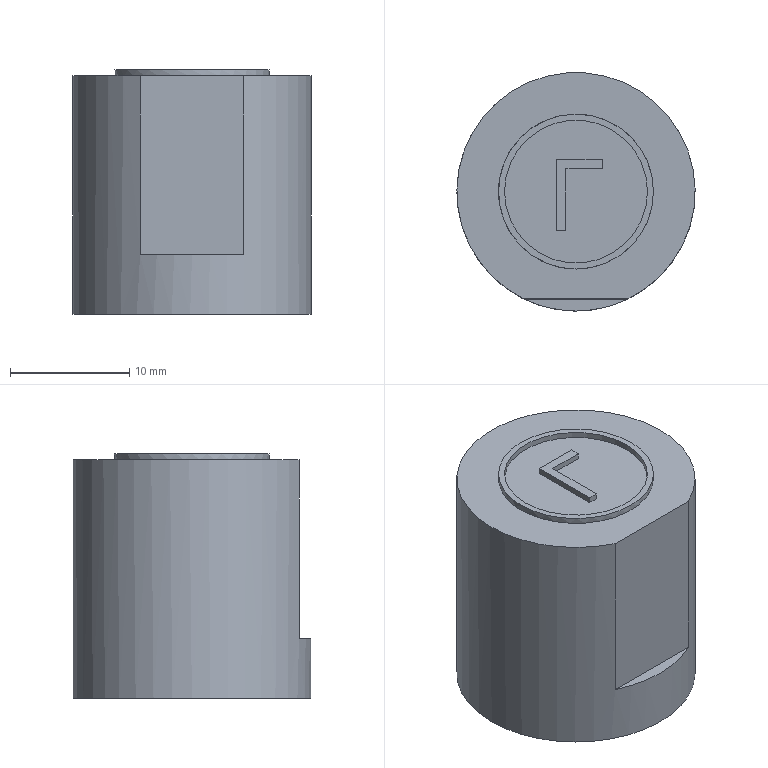Part | STEP file | lll_id694_x_t | 1 solid | 16 faces | box 20 x 20 x 20.5 mm | volume 6209 mm3 | plane 13 | cylinder 3 | commonest cylinder face diameters 12 x1 13 x1 20 x1
STEP:
#1=CARTESIAN_POINT('',(393.859,-109.,0.));
#2=VERTEX_POINT('',#1);
#3=CARTESIAN_POINT('',(385.141,-109.,0.));
#4=VERTEX_POINT('',#3);
#5=CARTESIAN_POINT('',(389.5,-109.,0.));
#6=DIRECTION('',(-1.,0.,0.));
#7=VECTOR('',#6,1.);
#8=LINE('',#5,#7);
#9=EDGE_CURVE('',#2,#4,#8,.T.);
#10=ORIENTED_EDGE('',*,*,#9,.F.);
#11=CARTESIAN_POINT('',(389.5,-100.,0.));
#12=DIRECTION('',(0.,0.,1.));
#13=DIRECTION('',(1.,0.,0.));
#14=AXIS2_PLACEMENT_3D('',#11,#12,#13);
#15=CIRCLE('',#14,10.);
#16=EDGE_CURVE('',#2,#4,#15,.T.);
#17=ORIENTED_EDGE('',*,*,#16,.T.);
#18=EDGE_LOOP('',(#10,#17));
#19=FACE_BOUND('',#18,.T.);
#20=CARTESIAN_POINT('',(396.,-100.,0.));
#21=VERTEX_POINT('',#20);
#22=CARTESIAN_POINT('',(389.5,-100.,0.));
#23=DIRECTION('',(0.,0.,-1.));
#24=DIRECTION('',(1.,0.,0.));
#25=AXIS2_PLACEMENT_3D('',#22,#23,#24);
#26=CIRCLE('',#25,6.5);
#27=EDGE_CURVE('',#21,#21,#26,.T.);
#28=ORIENTED_EDGE('',*,*,#27,.T.);
#29=EDGE_LOOP('',(#28));
#30=FACE_BOUND('',#29,.T.);
#31=CARTESIAN_POINT('',(389.5,-100.,0.));
#32=DIRECTION('',(0.,0.,1.));
#33=DIRECTION('',(1.,0.,0.));
#34=AXIS2_PLACEMENT_3D('',#31,#32,#33);
#35=PLANE('',#34);
#36=ADVANCED_FACE('',(#19,#30),#35,.T.);
#37=CARTESIAN_POINT('',(379.5,-100.,-20.));
#38=VERTEX_POINT('',#37);
#39=CARTESIAN_POINT('',(389.5,-100.,-20.));
#40=DIRECTION('',(0.,0.,1.));
#41=DIRECTION('',(-1.,0.,0.));
#42=AXIS2_PLACEMENT_3D('',#39,#40,#41);
#43=CIRCLE('',#42,10.);
#44=EDGE_CURVE('',#38,#38,#43,.T.);
#45=ORIENTED_EDGE('',*,*,#44,.T.);
#46=EDGE_LOOP('',(#45));
#47=FACE_BOUND('',#46,.T.);
#48=CARTESIAN_POINT('',(385.141,-109.,-15.));
#49=VERTEX_POINT('',#48);
#50=CARTESIAN_POINT('',(393.859,-109.,-15.));
#51=VERTEX_POINT('',#50);
#52=CARTESIAN_POINT('',(389.5,-100.,-15.));
#53=DIRECTION('',(0.,0.,1.));
#54=DIRECTION('',(1.,0.,0.));
#55=AXIS2_PLACEMENT_3D('',#52,#53,#54);
#56=CIRCLE('',#55,10.);
#57=EDGE_CURVE('',#49,#51,#56,.T.);
#58=ORIENTED_EDGE('',*,*,#57,.F.);
#59=CARTESIAN_POINT('',(385.141,-109.,0.));
#60=DIRECTION('',(0.,0.,1.));
#61=VECTOR('',#60,1.);
#62=LINE('',#59,#61);
#63=EDGE_CURVE('',#49,#4,#62,.T.);
#64=ORIENTED_EDGE('',*,*,#63,.T.);
#65=ORIENTED_EDGE('',*,*,#16,.F.);
#66=CARTESIAN_POINT('',(393.859,-109.,0.));
#67=DIRECTION('',(0.,0.,-1.));
#68=VECTOR('',#67,1.);
#69=LINE('',#66,#68);
#70=EDGE_CURVE('',#2,#51,#69,.T.);
#71=ORIENTED_EDGE('',*,*,#70,.T.);
#72=EDGE_LOOP('',(#58,#64,#65,#71));
#73=FACE_BOUND('',#72,.T.);
#74=CARTESIAN_POINT('',(389.5,-100.,0.));
#75=DIRECTION('',(0.,0.,-1.));
#76=DIRECTION('',(1.,0.,0.));
#77=AXIS2_PLACEMENT_3D('',#74,#75,#76);
#78=CYLINDRICAL_SURFACE('',#77,10.);
#79=ADVANCED_FACE('',(#47,#73),#78,.T.);
#80=ORIENTED_EDGE('',*,*,#70,.F.);
#81=ORIENTED_EDGE('',*,*,#9,.T.);
#82=ORIENTED_EDGE('',*,*,#63,.F.);
#83=CARTESIAN_POINT('',(393.623,-109.,-15.));
#84=DIRECTION('',(-1.,0.,0.));
#85=VECTOR('',#84,1.);
#86=LINE('',#83,#85);
#87=EDGE_CURVE('',#51,#49,#86,.T.);
#88=ORIENTED_EDGE('',*,*,#87,.F.);
#89=EDGE_LOOP('',(#80,#81,#82,#88));
#90=FACE_OUTER_BOUND('',#89,.T.);
#91=CARTESIAN_POINT('',(389.5,-109.,-10.));
#92=DIRECTION('',(0.,1.,0.));
#93=DIRECTION('',(0.,0.,1.));
#94=AXIS2_PLACEMENT_3D('',#91,#92,#93);
#95=PLANE('',#94);
#96=ADVANCED_FACE('',(#90),#95,.F.);
#97=ORIENTED_EDGE('',*,*,#44,.F.);
#98=EDGE_LOOP('',(#97));
#99=FACE_OUTER_BOUND('',#98,.T.);
#100=CARTESIAN_POINT('',(389.5,-100.,-20.));
#101=DIRECTION('',(0.,0.,-1.));
#102=DIRECTION('',(-1.,0.,0.));
#103=AXIS2_PLACEMENT_3D('',#100,#101,#102);
#104=PLANE('',#103);
#105=ADVANCED_FACE('',(#99),#104,.T.);
#106=ORIENTED_EDGE('',*,*,#87,.T.);
#107=ORIENTED_EDGE('',*,*,#57,.T.);
#108=EDGE_LOOP('',(#106,#107));
#109=FACE_OUTER_BOUND('',#108,.T.);
#110=CARTESIAN_POINT('',(393.623,-114.35,-15.));
#111=DIRECTION('',(0.,0.,1.));
#112=DIRECTION('',(-1.,0.,0.));
#113=AXIS2_PLACEMENT_3D('',#110,#111,#112);
#114=PLANE('',#113);
#115=ADVANCED_FACE('',(#109),#114,.T.);
#116=ORIENTED_EDGE('',*,*,#27,.F.);
#117=EDGE_LOOP('',(#116));
#118=FACE_BOUND('',#117,.T.);
#119=CARTESIAN_POINT('',(383.,-100.,0.5));
#120=VERTEX_POINT('',#119);
#121=CARTESIAN_POINT('',(389.5,-100.,0.5));
#122=DIRECTION('',(0.,0.,1.));
#123=DIRECTION('',(-1.,0.,0.));
#124=AXIS2_PLACEMENT_3D('',#121,#122,#123);
#125=CIRCLE('',#124,6.5);
#126=EDGE_CURVE('',#120,#120,#125,.T.);
#127=ORIENTED_EDGE('',*,*,#126,.F.);
#128=EDGE_LOOP('',(#127));
#129=FACE_BOUND('',#128,.T.);
#130=CARTESIAN_POINT('',(389.5,-100.,-2.));
#131=DIRECTION('',(0.,0.,1.));
#132=DIRECTION('',(1.,0.,0.));
#133=AXIS2_PLACEMENT_3D('',#130,#131,#132);
#134=CYLINDRICAL_SURFACE('',#133,6.5);
#135=ADVANCED_FACE('',(#118,#129),#134,.T.);
#136=ORIENTED_EDGE('',*,*,#126,.T.);
#137=EDGE_LOOP('',(#136));
#138=FACE_BOUND('',#137,.T.);
#139=CARTESIAN_POINT('',(383.5,-100.,0.5));
#140=VERTEX_POINT('',#139);
#141=CARTESIAN_POINT('',(389.5,-100.,0.5));
#142=DIRECTION('',(0.,0.,1.));
#143=DIRECTION('',(-1.,0.,0.));
#144=AXIS2_PLACEMENT_3D('',#141,#142,#143);
#145=CIRCLE('',#144,6.);
#146=EDGE_CURVE('',#140,#140,#145,.T.);
#147=ORIENTED_EDGE('',*,*,#146,.F.);
#148=EDGE_LOOP('',(#147));
#149=FACE_BOUND('',#148,.T.);
#150=CARTESIAN_POINT('',(389.5,-100.,0.5));
#151=DIRECTION('',(0.,0.,1.));
#152=DIRECTION('',(1.,0.,0.));
#153=AXIS2_PLACEMENT_3D('',#150,#151,#152);
#154=PLANE('',#153);
#155=ADVANCED_FACE('',(#138,#149),#154,.T.);
#156=CARTESIAN_POINT('',(395.5,-100.,0.));
#157=VERTEX_POINT('',#156);
#158=CARTESIAN_POINT('',(389.5,-100.,0.));
#159=DIRECTION('',(0.,0.,1.));
#160=DIRECTION('',(1.,0.,0.));
#161=AXIS2_PLACEMENT_3D('',#158,#159,#160);
#162=CIRCLE('',#161,6.);
#163=EDGE_CURVE('',#157,#157,#162,.T.);
#164=ORIENTED_EDGE('',*,*,#163,.F.);
#165=EDGE_LOOP('',(#164));
#166=FACE_BOUND('',#165,.T.);
#167=ORIENTED_EDGE('',*,*,#146,.T.);
#168=EDGE_LOOP('',(#167));
#169=FACE_BOUND('',#168,.T.);
#170=CARTESIAN_POINT('',(389.5,-100.,-2.));
#171=DIRECTION('',(0.,0.,1.));
#172=DIRECTION('',(1.,0.,0.));
#173=AXIS2_PLACEMENT_3D('',#170,#171,#172);
#174=CYLINDRICAL_SURFACE('',#173,6.);
#175=ADVANCED_FACE('',(#166,#169),#174,.F.);
#176=CARTESIAN_POINT('',(388.657,-103.274,0.5));
#177=VERTEX_POINT('',#176);
#178=CARTESIAN_POINT('',(387.857,-103.274,0.5));
#179=VERTEX_POINT('',#178);
#180=CARTESIAN_POINT('',(388.257,-103.274,0.5));
#181=DIRECTION('',(-1.,0.,0.));
#182=VECTOR('',#181,1.);
#183=LINE('',#180,#182);
#184=EDGE_CURVE('',#177,#179,#183,.T.);
#185=ORIENTED_EDGE('',*,*,#184,.F.);
#186=CARTESIAN_POINT('',(388.657,-98.074,0.5));
#187=VERTEX_POINT('',#186);
#188=CARTESIAN_POINT('',(388.657,-100.674,0.5));
#189=DIRECTION('',(0.,-1.,0.));
#190=VECTOR('',#189,1.);
#191=LINE('',#188,#190);
#192=EDGE_CURVE('',#187,#177,#191,.T.);
#193=ORIENTED_EDGE('',*,*,#192,.F.);
#194=CARTESIAN_POINT('',(391.707,-98.074,0.5));
#195=VERTEX_POINT('',#194);
#196=CARTESIAN_POINT('',(390.182,-98.074,0.5));
#197=DIRECTION('',(-1.,0.,0.));
#198=VECTOR('',#197,1.);
#199=LINE('',#196,#198);
#200=EDGE_CURVE('',#195,#187,#199,.T.);
#201=ORIENTED_EDGE('',*,*,#200,.F.);
#202=CARTESIAN_POINT('',(391.707,-97.274,0.5));
#203=VERTEX_POINT('',#202);
#204=CARTESIAN_POINT('',(391.707,-97.674,0.5));
#205=DIRECTION('',(0.,-1.,0.));
#206=VECTOR('',#205,1.);
#207=LINE('',#204,#206);
#208=EDGE_CURVE('',#203,#195,#207,.T.);
#209=ORIENTED_EDGE('',*,*,#208,.F.);
#210=CARTESIAN_POINT('',(387.857,-97.274,0.5));
#211=VERTEX_POINT('',#210);
#212=CARTESIAN_POINT('',(389.782,-97.274,0.5));
#213=DIRECTION('',(1.,0.,0.));
#214=VECTOR('',#213,1.);
#215=LINE('',#212,#214);
#216=EDGE_CURVE('',#211,#203,#215,.T.);
#217=ORIENTED_EDGE('',*,*,#216,.F.);
#218=CARTESIAN_POINT('',(387.857,-100.274,0.5));
#219=DIRECTION('',(0.,1.,0.));
#220=VECTOR('',#219,1.);
#221=LINE('',#218,#220);
#222=EDGE_CURVE('',#179,#211,#221,.T.);
#223=ORIENTED_EDGE('',*,*,#222,.F.);
#224=EDGE_LOOP('',(#185,#193,#201,#209,#217,#223));
#225=FACE_OUTER_BOUND('',#224,.T.);
#226=CARTESIAN_POINT('',(388.257,-103.274,0.5));
#227=DIRECTION('',(0.,0.,1.));
#228=DIRECTION('',(1.,0.,0.));
#229=AXIS2_PLACEMENT_3D('',#226,#227,#228);
#230=PLANE('',#229);
#231=ADVANCED_FACE('',(#225),#230,.T.);
#232=CARTESIAN_POINT('',(388.657,-103.274,0.));
#233=VERTEX_POINT('',#232);
#234=CARTESIAN_POINT('',(388.657,-103.274,-2.));
#235=DIRECTION('',(0.,0.,1.));
#236=VECTOR('',#235,1.);
#237=LINE('',#234,#236);
#238=EDGE_CURVE('',#233,#177,#237,.T.);
#239=ORIENTED_EDGE('',*,*,#238,.F.);
#240=CARTESIAN_POINT('',(388.657,-98.074,0.));
#241=VERTEX_POINT('',#240);
#242=CARTESIAN_POINT('',(388.657,-98.074,0.));
#243=DIRECTION('',(0.,1.,0.));
#244=VECTOR('',#243,1.);
#245=LINE('',#242,#244);
#246=EDGE_CURVE('',#233,#241,#245,.T.);
#247=ORIENTED_EDGE('',*,*,#246,.T.);
#248=CARTESIAN_POINT('',(388.657,-98.074,-2.));
#249=DIRECTION('',(0.,0.,1.));
#250=VECTOR('',#249,1.);
#251=LINE('',#248,#250);
#252=EDGE_CURVE('',#241,#187,#251,.T.);
#253=ORIENTED_EDGE('',*,*,#252,.T.);
#254=ORIENTED_EDGE('',*,*,#192,.T.);
#255=EDGE_LOOP('',(#239,#247,#253,#254));
#256=FACE_OUTER_BOUND('',#255,.T.);
#257=CARTESIAN_POINT('',(388.657,-98.074,-2.));
#258=DIRECTION('',(-1.,0.,0.));
#259=DIRECTION('',(0.,0.,1.));
#260=AXIS2_PLACEMENT_3D('',#257,#258,#259);
#261=PLANE('',#260);
#262=ADVANCED_FACE('',(#256),#261,.F.);
#263=ORIENTED_EDGE('',*,*,#252,.F.);
#264=CARTESIAN_POINT('',(391.707,-98.074,0.));
#265=VERTEX_POINT('',#264);
#266=CARTESIAN_POINT('',(391.707,-98.074,0.));
#267=DIRECTION('',(-1.,0.,0.));
#268=VECTOR('',#267,1.);
#269=LINE('',#266,#268);
#270=EDGE_CURVE('',#265,#241,#269,.T.);
#271=ORIENTED_EDGE('',*,*,#270,.F.);
#272=CARTESIAN_POINT('',(391.707,-98.074,-2.));
#273=DIRECTION('',(0.,0.,1.));
#274=VECTOR('',#273,1.);
#275=LINE('',#272,#274);
#276=EDGE_CURVE('',#265,#195,#275,.T.);
#277=ORIENTED_EDGE('',*,*,#276,.T.);
#278=ORIENTED_EDGE('',*,*,#200,.T.);
#279=EDGE_LOOP('',(#263,#271,#277,#278));
#280=FACE_OUTER_BOUND('',#279,.T.);
#281=CARTESIAN_POINT('',(391.707,-98.074,-2.));
#282=DIRECTION('',(0.,1.,0.));
#283=DIRECTION('',(0.,0.,1.));
#284=AXIS2_PLACEMENT_3D('',#281,#282,#283);
#285=PLANE('',#284);
#286=ADVANCED_FACE('',(#280),#285,.F.);
#287=ORIENTED_EDGE('',*,*,#276,.F.);
#288=CARTESIAN_POINT('',(391.707,-97.274,0.));
#289=VERTEX_POINT('',#288);
#290=CARTESIAN_POINT('',(391.707,-97.274,0.));
#291=DIRECTION('',(0.,1.,0.));
#292=VECTOR('',#291,1.);
#293=LINE('',#290,#292);
#294=EDGE_CURVE('',#265,#289,#293,.T.);
#295=ORIENTED_EDGE('',*,*,#294,.T.);
#296=CARTESIAN_POINT('',(391.707,-97.274,-2.));
#297=DIRECTION('',(0.,0.,1.));
#298=VECTOR('',#297,1.);
#299=LINE('',#296,#298);
#300=EDGE_CURVE('',#289,#203,#299,.T.);
#301=ORIENTED_EDGE('',*,*,#300,.T.);
#302=ORIENTED_EDGE('',*,*,#208,.T.);
#303=EDGE_LOOP('',(#287,#295,#301,#302));
#304=FACE_OUTER_BOUND('',#303,.T.);
#305=CARTESIAN_POINT('',(391.707,-97.274,-2.));
#306=DIRECTION('',(-1.,0.,0.));
#307=DIRECTION('',(0.,0.,1.));
#308=AXIS2_PLACEMENT_3D('',#305,#306,#307);
#309=PLANE('',#308);
#310=ADVANCED_FACE('',(#304),#309,.F.);
#311=ORIENTED_EDGE('',*,*,#300,.F.);
#312=CARTESIAN_POINT('',(387.857,-97.274,0.));
#313=VERTEX_POINT('',#312);
#314=CARTESIAN_POINT('',(387.857,-97.274,0.));
#315=DIRECTION('',(-1.,0.,0.));
#316=VECTOR('',#315,1.);
#317=LINE('',#314,#316);
#318=EDGE_CURVE('',#289,#313,#317,.T.);
#319=ORIENTED_EDGE('',*,*,#318,.T.);
#320=CARTESIAN_POINT('',(387.857,-97.274,-2.));
#321=DIRECTION('',(0.,0.,1.));
#322=VECTOR('',#321,1.);
#323=LINE('',#320,#322);
#324=EDGE_CURVE('',#313,#211,#323,.T.);
#325=ORIENTED_EDGE('',*,*,#324,.T.);
#326=ORIENTED_EDGE('',*,*,#216,.T.);
#327=EDGE_LOOP('',(#311,#319,#325,#326));
#328=FACE_OUTER_BOUND('',#327,.T.);
#329=CARTESIAN_POINT('',(387.857,-97.274,-2.));
#330=DIRECTION('',(0.,-1.,0.));
#331=DIRECTION('',(0.,0.,-1.));
#332=AXIS2_PLACEMENT_3D('',#329,#330,#331);
#333=PLANE('',#332);
#334=ADVANCED_FACE('',(#328),#333,.F.);
#335=ORIENTED_EDGE('',*,*,#324,.F.);
#336=CARTESIAN_POINT('',(387.857,-103.274,0.));
#337=VERTEX_POINT('',#336);
#338=CARTESIAN_POINT('',(387.857,-103.274,0.));
#339=DIRECTION('',(0.,-1.,0.));
#340=VECTOR('',#339,1.);
#341=LINE('',#338,#340);
#342=EDGE_CURVE('',#313,#337,#341,.T.);
#343=ORIENTED_EDGE('',*,*,#342,.T.);
#344=CARTESIAN_POINT('',(387.857,-103.274,-2.));
#345=DIRECTION('',(0.,0.,1.));
#346=VECTOR('',#345,1.);
#347=LINE('',#344,#346);
#348=EDGE_CURVE('',#337,#179,#347,.T.);
#349=ORIENTED_EDGE('',*,*,#348,.T.);
#350=ORIENTED_EDGE('',*,*,#222,.T.);
#351=EDGE_LOOP('',(#335,#343,#349,#350));
#352=FACE_OUTER_BOUND('',#351,.T.);
#353=CARTESIAN_POINT('',(387.857,-103.274,-2.));
#354=DIRECTION('',(1.,0.,0.));
#355=DIRECTION('',(0.,0.,-1.));
#356=AXIS2_PLACEMENT_3D('',#353,#354,#355);
#357=PLANE('',#356);
#358=ADVANCED_FACE('',(#352),#357,.F.);
#359=ORIENTED_EDGE('',*,*,#348,.F.);
#360=CARTESIAN_POINT('',(388.657,-103.274,0.));
#361=DIRECTION('',(1.,0.,0.));
#362=VECTOR('',#361,1.);
#363=LINE('',#360,#362);
#364=EDGE_CURVE('',#337,#233,#363,.T.);
#365=ORIENTED_EDGE('',*,*,#364,.T.);
#366=ORIENTED_EDGE('',*,*,#238,.T.);
#367=ORIENTED_EDGE('',*,*,#184,.T.);
#368=EDGE_LOOP('',(#359,#365,#366,#367));
#369=FACE_OUTER_BOUND('',#368,.T.);
#370=CARTESIAN_POINT('',(388.657,-103.274,-2.));
#371=DIRECTION('',(0.,1.,0.));
#372=DIRECTION('',(0.,0.,1.));
#373=AXIS2_PLACEMENT_3D('',#370,#371,#372);
#374=PLANE('',#373);
#375=ADVANCED_FACE('',(#369),#374,.F.);
#376=ORIENTED_EDGE('',*,*,#364,.F.);
#377=ORIENTED_EDGE('',*,*,#342,.F.);
#378=ORIENTED_EDGE('',*,*,#318,.F.);
#379=ORIENTED_EDGE('',*,*,#294,.F.);
#380=ORIENTED_EDGE('',*,*,#270,.T.);
#381=ORIENTED_EDGE('',*,*,#246,.F.);
#382=EDGE_LOOP('',(#376,#377,#378,#379,#380,#381));
#383=FACE_BOUND('',#382,.T.);
#384=ORIENTED_EDGE('',*,*,#163,.T.);
#385=EDGE_LOOP('',(#384));
#386=FACE_BOUND('',#385,.T.);
#387=CARTESIAN_POINT('',(389.5,-100.,0.));
#388=DIRECTION('',(0.,0.,1.));
#389=DIRECTION('',(1.,0.,0.));
#390=AXIS2_PLACEMENT_3D('',#387,#388,#389);
#391=PLANE('',#390);
#392=ADVANCED_FACE('',(#383,#386),#391,.T.);
#393=CLOSED_SHELL('',(#36,#79,#96,#105,#115,#135,#155,#175,#231,#262,#286,#310,#334,#358,#375,#392));
#394=MANIFOLD_SOLID_BREP('',#393);
#395=(LENGTH_UNIT()NAMED_UNIT(*)SI_UNIT(.MILLI.,.METRE.));
#396=UNCERTAINTY_MEASURE_WITH_UNIT(LENGTH_MEASURE(0.00002),#395,'','');
#397=(NAMED_UNIT(*)PLANE_ANGLE_UNIT()SI_UNIT($,.RADIAN.));
#398=PLANE_ANGLE_MEASURE_WITH_UNIT(PLANE_ANGLE_MEASURE(0.01745),#397);
#399=DIMENSIONAL_EXPONENTS(0.,0.,0.,0.,0.,0.,0.);
#400=(CONVERSION_BASED_UNIT('DEGREE',#398)NAMED_UNIT(#399)PLANE_ANGLE_UNIT());
#401=(NAMED_UNIT(*)SI_UNIT($,.STERADIAN.)SOLID_ANGLE_UNIT());
#402=(GEOMETRIC_REPRESENTATION_CONTEXT(3)GLOBAL_UNCERTAINTY_ASSIGNED_CONTEXT((#396))GLOBAL_UNIT_ASSIGNED_CONTEXT((#395,#400,#401))REPRESENTATION_CONTEXT('',''));
#403=ADVANCED_BREP_SHAPE_REPRESENTATION('',(#394),#402);